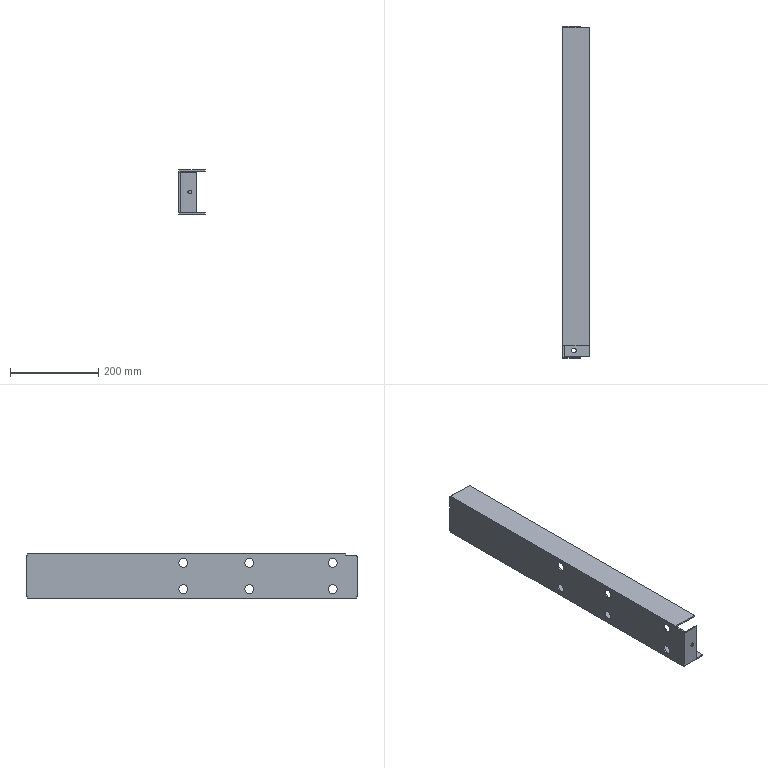Part | SolidWorks | features BaseBody 1 | 1 solid | 44 faces | box 60 x 754 x 100 mm | volume 491228 mm3 | plane 24 | cylinder 20 | commonest cylinder face diameters 20 x12 11 x4 8.5 x2 10.6 x2
STEP:
#1=CARTESIAN_POINT('',(199.946,-4340.973,914.971));
#2=VERTEX_POINT('',#1);
#3=CARTESIAN_POINT('',(199.946,-4340.973,934.971));
#4=VERTEX_POINT('',#3);
#5=CARTESIAN_POINT('',(199.946,-4340.973,924.971));
#6=DIRECTION('',(-1.,0.,0.));
#7=DIRECTION('',(0.,0.,1.));
#8=AXIS2_PLACEMENT_3D('',#5,#6,#7);
#9=CIRCLE('',#8,10.);
#10=EDGE_CURVE('',#2,#4,#9,.T.);
#11=ORIENTED_EDGE('',*,*,#10,.F.);
#12=CARTESIAN_POINT('',(196.946,-4340.973,914.971));
#13=VERTEX_POINT('',#12);
#14=CARTESIAN_POINT('',(218.146,-4340.973,914.971));
#15=DIRECTION('',(-1.,0.,0.));
#16=VECTOR('',#15,1000.);
#17=LINE('',#14,#16);
#18=EDGE_CURVE('',#2,#13,#17,.T.);
#19=ORIENTED_EDGE('',*,*,#18,.T.);
#20=CARTESIAN_POINT('',(196.946,-4340.973,934.971));
#21=VERTEX_POINT('',#20);
#22=CARTESIAN_POINT('',(196.946,-4340.973,924.971));
#23=DIRECTION('',(1.,0.,0.));
#24=DIRECTION('',(0.,0.,1.));
#25=AXIS2_PLACEMENT_3D('',#22,#23,#24);
#26=CIRCLE('',#25,10.);
#27=EDGE_CURVE('',#21,#13,#26,.T.);
#28=ORIENTED_EDGE('',*,*,#27,.F.);
#29=CARTESIAN_POINT('',(218.146,-4340.973,934.971));
#30=DIRECTION('',(-1.,0.,0.));
#31=VECTOR('',#30,1000.);
#32=LINE('',#29,#31);
#33=EDGE_CURVE('',#4,#21,#32,.T.);
#34=ORIENTED_EDGE('',*,*,#33,.F.);
#35=EDGE_LOOP('',(#11,#19,#28,#34));
#36=FACE_OUTER_BOUND('',#35,.T.);
#37=CARTESIAN_POINT('',(218.146,-4340.973,924.971));
#38=DIRECTION('',(-1.,0.,0.));
#39=DIRECTION('',(0.,0.,1.));
#40=AXIS2_PLACEMENT_3D('',#37,#38,#39);
#41=CYLINDRICAL_SURFACE('',#40,10.);
#42=ADVANCED_FACE('',(#36),#41,.F.);
#43=CARTESIAN_POINT('',(199.946,-4150.973,854.971));
#44=VERTEX_POINT('',#43);
#45=CARTESIAN_POINT('',(199.946,-4150.973,874.971));
#46=VERTEX_POINT('',#45);
#47=CARTESIAN_POINT('',(199.946,-4150.973,864.971));
#48=DIRECTION('',(-1.,0.,0.));
#49=DIRECTION('',(0.,0.,1.));
#50=AXIS2_PLACEMENT_3D('',#47,#48,#49);
#51=CIRCLE('',#50,10.);
#52=EDGE_CURVE('',#44,#46,#51,.T.);
#53=ORIENTED_EDGE('',*,*,#52,.F.);
#54=CARTESIAN_POINT('',(196.946,-4150.973,854.971));
#55=VERTEX_POINT('',#54);
#56=CARTESIAN_POINT('',(218.146,-4150.973,854.971));
#57=DIRECTION('',(-1.,0.,0.));
#58=VECTOR('',#57,1000.);
#59=LINE('',#56,#58);
#60=EDGE_CURVE('',#44,#55,#59,.T.);
#61=ORIENTED_EDGE('',*,*,#60,.T.);
#62=CARTESIAN_POINT('',(196.946,-4150.973,874.971));
#63=VERTEX_POINT('',#62);
#64=CARTESIAN_POINT('',(196.946,-4150.973,864.971));
#65=DIRECTION('',(1.,0.,0.));
#66=DIRECTION('',(0.,0.,1.));
#67=AXIS2_PLACEMENT_3D('',#64,#65,#66);
#68=CIRCLE('',#67,10.);
#69=EDGE_CURVE('',#63,#55,#68,.T.);
#70=ORIENTED_EDGE('',*,*,#69,.F.);
#71=CARTESIAN_POINT('',(218.146,-4150.973,874.971));
#72=DIRECTION('',(-1.,0.,0.));
#73=VECTOR('',#72,1000.);
#74=LINE('',#71,#73);
#75=EDGE_CURVE('',#46,#63,#74,.T.);
#76=ORIENTED_EDGE('',*,*,#75,.F.);
#77=EDGE_LOOP('',(#53,#61,#70,#76));
#78=FACE_OUTER_BOUND('',#77,.T.);
#79=CARTESIAN_POINT('',(218.146,-4150.973,864.971));
#80=DIRECTION('',(-1.,0.,0.));
#81=DIRECTION('',(0.,0.,1.));
#82=AXIS2_PLACEMENT_3D('',#79,#80,#81);
#83=CYLINDRICAL_SURFACE('',#82,10.);
#84=ADVANCED_FACE('',(#78),#83,.F.);
#85=CARTESIAN_POINT('',(199.946,-4000.973,914.971));
#86=VERTEX_POINT('',#85);
#87=CARTESIAN_POINT('',(199.946,-4000.973,934.971));
#88=VERTEX_POINT('',#87);
#89=CARTESIAN_POINT('',(199.946,-4000.973,924.971));
#90=DIRECTION('',(-1.,0.,0.));
#91=DIRECTION('',(0.,0.,1.));
#92=AXIS2_PLACEMENT_3D('',#89,#90,#91);
#93=CIRCLE('',#92,10.);
#94=EDGE_CURVE('',#86,#88,#93,.T.);
#95=ORIENTED_EDGE('',*,*,#94,.F.);
#96=CARTESIAN_POINT('',(196.946,-4000.973,914.971));
#97=VERTEX_POINT('',#96);
#98=CARTESIAN_POINT('',(218.146,-4000.973,914.971));
#99=DIRECTION('',(-1.,0.,0.));
#100=VECTOR('',#99,1000.);
#101=LINE('',#98,#100);
#102=EDGE_CURVE('',#86,#97,#101,.T.);
#103=ORIENTED_EDGE('',*,*,#102,.T.);
#104=CARTESIAN_POINT('',(196.946,-4000.973,934.971));
#105=VERTEX_POINT('',#104);
#106=CARTESIAN_POINT('',(196.946,-4000.973,924.971));
#107=DIRECTION('',(1.,0.,0.));
#108=DIRECTION('',(0.,0.,1.));
#109=AXIS2_PLACEMENT_3D('',#106,#107,#108);
#110=CIRCLE('',#109,10.);
#111=EDGE_CURVE('',#105,#97,#110,.T.);
#112=ORIENTED_EDGE('',*,*,#111,.F.);
#113=CARTESIAN_POINT('',(218.146,-4000.973,934.971));
#114=DIRECTION('',(-1.,0.,0.));
#115=VECTOR('',#114,1000.);
#116=LINE('',#113,#115);
#117=EDGE_CURVE('',#88,#105,#116,.T.);
#118=ORIENTED_EDGE('',*,*,#117,.F.);
#119=EDGE_LOOP('',(#95,#103,#112,#118));
#120=FACE_OUTER_BOUND('',#119,.T.);
#121=CARTESIAN_POINT('',(218.146,-4000.973,924.971));
#122=DIRECTION('',(-1.,0.,0.));
#123=DIRECTION('',(0.,0.,1.));
#124=AXIS2_PLACEMENT_3D('',#121,#122,#123);
#125=CYLINDRICAL_SURFACE('',#124,10.);
#126=ADVANCED_FACE('',(#120),#125,.F.);
#127=CARTESIAN_POINT('',(199.946,-4000.973,854.971));
#128=VERTEX_POINT('',#127);
#129=CARTESIAN_POINT('',(199.946,-4000.973,874.971));
#130=VERTEX_POINT('',#129);
#131=CARTESIAN_POINT('',(199.946,-4000.973,864.971));
#132=DIRECTION('',(-1.,0.,0.));
#133=DIRECTION('',(0.,0.,1.));
#134=AXIS2_PLACEMENT_3D('',#131,#132,#133);
#135=CIRCLE('',#134,10.);
#136=EDGE_CURVE('',#128,#130,#135,.T.);
#137=ORIENTED_EDGE('',*,*,#136,.F.);
#138=CARTESIAN_POINT('',(196.946,-4000.973,854.971));
#139=VERTEX_POINT('',#138);
#140=CARTESIAN_POINT('',(218.146,-4000.973,854.971));
#141=DIRECTION('',(-1.,0.,0.));
#142=VECTOR('',#141,1000.);
#143=LINE('',#140,#142);
#144=EDGE_CURVE('',#128,#139,#143,.T.);
#145=ORIENTED_EDGE('',*,*,#144,.T.);
#146=CARTESIAN_POINT('',(196.946,-4000.973,874.971));
#147=VERTEX_POINT('',#146);
#148=CARTESIAN_POINT('',(196.946,-4000.973,864.971));
#149=DIRECTION('',(1.,0.,0.));
#150=DIRECTION('',(0.,0.,1.));
#151=AXIS2_PLACEMENT_3D('',#148,#149,#150);
#152=CIRCLE('',#151,10.);
#153=EDGE_CURVE('',#147,#139,#152,.T.);
#154=ORIENTED_EDGE('',*,*,#153,.F.);
#155=CARTESIAN_POINT('',(218.146,-4000.973,874.971));
#156=DIRECTION('',(-1.,0.,0.));
#157=VECTOR('',#156,1000.);
#158=LINE('',#155,#157);
#159=EDGE_CURVE('',#130,#147,#158,.T.);
#160=ORIENTED_EDGE('',*,*,#159,.F.);
#161=EDGE_LOOP('',(#137,#145,#154,#160));
#162=FACE_OUTER_BOUND('',#161,.T.);
#163=CARTESIAN_POINT('',(218.146,-4000.973,864.971));
#164=DIRECTION('',(-1.,0.,0.));
#165=DIRECTION('',(0.,0.,1.));
#166=AXIS2_PLACEMENT_3D('',#163,#164,#165);
#167=CYLINDRICAL_SURFACE('',#166,10.);
#168=ADVANCED_FACE('',(#162),#167,.F.);
#169=CARTESIAN_POINT('',(199.946,-4150.973,914.971));
#170=VERTEX_POINT('',#169);
#171=CARTESIAN_POINT('',(199.946,-4150.973,934.971));
#172=VERTEX_POINT('',#171);
#173=CARTESIAN_POINT('',(199.946,-4150.973,924.971));
#174=DIRECTION('',(-1.,0.,0.));
#175=DIRECTION('',(0.,0.,1.));
#176=AXIS2_PLACEMENT_3D('',#173,#174,#175);
#177=CIRCLE('',#176,10.);
#178=EDGE_CURVE('',#170,#172,#177,.T.);
#179=ORIENTED_EDGE('',*,*,#178,.F.);
#180=CARTESIAN_POINT('',(196.946,-4150.973,914.971));
#181=VERTEX_POINT('',#180);
#182=CARTESIAN_POINT('',(218.146,-4150.973,914.971));
#183=DIRECTION('',(-1.,0.,0.));
#184=VECTOR('',#183,1000.);
#185=LINE('',#182,#184);
#186=EDGE_CURVE('',#170,#181,#185,.T.);
#187=ORIENTED_EDGE('',*,*,#186,.T.);
#188=CARTESIAN_POINT('',(196.946,-4150.973,934.971));
#189=VERTEX_POINT('',#188);
#190=CARTESIAN_POINT('',(196.946,-4150.973,924.971));
#191=DIRECTION('',(1.,0.,0.));
#192=DIRECTION('',(0.,0.,1.));
#193=AXIS2_PLACEMENT_3D('',#190,#191,#192);
#194=CIRCLE('',#193,10.);
#195=EDGE_CURVE('',#189,#181,#194,.T.);
#196=ORIENTED_EDGE('',*,*,#195,.F.);
#197=CARTESIAN_POINT('',(218.146,-4150.973,934.971));
#198=DIRECTION('',(-1.,0.,0.));
#199=VECTOR('',#198,1000.);
#200=LINE('',#197,#199);
#201=EDGE_CURVE('',#172,#189,#200,.T.);
#202=ORIENTED_EDGE('',*,*,#201,.F.);
#203=EDGE_LOOP('',(#179,#187,#196,#202));
#204=FACE_OUTER_BOUND('',#203,.T.);
#205=CARTESIAN_POINT('',(218.146,-4150.973,924.971));
#206=DIRECTION('',(-1.,0.,0.));
#207=DIRECTION('',(0.,0.,1.));
#208=AXIS2_PLACEMENT_3D('',#205,#206,#207);
#209=CYLINDRICAL_SURFACE('',#208,10.);
#210=ADVANCED_FACE('',(#204),#209,.F.);
#211=CARTESIAN_POINT('',(199.946,-4340.973,854.971));
#212=VERTEX_POINT('',#211);
#213=CARTESIAN_POINT('',(199.946,-4340.973,874.971));
#214=VERTEX_POINT('',#213);
#215=CARTESIAN_POINT('',(199.946,-4340.973,864.971));
#216=DIRECTION('',(-1.,0.,0.));
#217=DIRECTION('',(0.,0.,1.));
#218=AXIS2_PLACEMENT_3D('',#215,#216,#217);
#219=CIRCLE('',#218,10.);
#220=EDGE_CURVE('',#212,#214,#219,.T.);
#221=ORIENTED_EDGE('',*,*,#220,.F.);
#222=CARTESIAN_POINT('',(196.946,-4340.973,854.971));
#223=VERTEX_POINT('',#222);
#224=CARTESIAN_POINT('',(218.146,-4340.973,854.971));
#225=DIRECTION('',(-1.,0.,0.));
#226=VECTOR('',#225,1000.);
#227=LINE('',#224,#226);
#228=EDGE_CURVE('',#212,#223,#227,.T.);
#229=ORIENTED_EDGE('',*,*,#228,.T.);
#230=CARTESIAN_POINT('',(196.946,-4340.973,874.971));
#231=VERTEX_POINT('',#230);
#232=CARTESIAN_POINT('',(196.946,-4340.973,864.971));
#233=DIRECTION('',(1.,0.,0.));
#234=DIRECTION('',(0.,0.,1.));
#235=AXIS2_PLACEMENT_3D('',#232,#233,#234);
#236=CIRCLE('',#235,10.);
#237=EDGE_CURVE('',#231,#223,#236,.T.);
#238=ORIENTED_EDGE('',*,*,#237,.F.);
#239=CARTESIAN_POINT('',(218.146,-4340.973,874.971));
#240=DIRECTION('',(-1.,0.,0.));
#241=VECTOR('',#240,1000.);
#242=LINE('',#239,#241);
#243=EDGE_CURVE('',#214,#231,#242,.T.);
#244=ORIENTED_EDGE('',*,*,#243,.F.);
#245=EDGE_LOOP('',(#221,#229,#238,#244));
#246=FACE_OUTER_BOUND('',#245,.T.);
#247=CARTESIAN_POINT('',(218.146,-4340.973,864.971));
#248=DIRECTION('',(-1.,0.,0.));
#249=DIRECTION('',(0.,0.,1.));
#250=AXIS2_PLACEMENT_3D('',#247,#248,#249);
#251=CYLINDRICAL_SURFACE('',#250,10.);
#252=ADVANCED_FACE('',(#246),#251,.F.);
#253=CARTESIAN_POINT('',(221.946,-4394.973,899.221));
#254=VERTEX_POINT('',#253);
#255=CARTESIAN_POINT('',(221.946,-4394.973,890.721));
#256=VERTEX_POINT('',#255);
#257=CARTESIAN_POINT('',(221.946,-4394.973,894.971));
#258=DIRECTION('',(0.,-1.,0.));
#259=DIRECTION('',(0.,0.,-1.));
#260=AXIS2_PLACEMENT_3D('',#257,#258,#259);
#261=CIRCLE('',#260,4.25);
#262=EDGE_CURVE('',#254,#256,#261,.T.);
#263=ORIENTED_EDGE('',*,*,#262,.F.);
#264=CARTESIAN_POINT('',(221.946,-4397.973,899.221));
#265=VERTEX_POINT('',#264);
#266=CARTESIAN_POINT('',(221.946,-4409.781,899.221));
#267=DIRECTION('',(0.,-1.,0.));
#268=VECTOR('',#267,1000.);
#269=LINE('',#266,#268);
#270=EDGE_CURVE('',#254,#265,#269,.T.);
#271=ORIENTED_EDGE('',*,*,#270,.T.);
#272=CARTESIAN_POINT('',(221.946,-4397.973,890.721));
#273=VERTEX_POINT('',#272);
#274=CARTESIAN_POINT('',(221.946,-4397.973,894.971));
#275=DIRECTION('',(0.,1.,0.));
#276=DIRECTION('',(0.,0.,-1.));
#277=AXIS2_PLACEMENT_3D('',#274,#275,#276);
#278=CIRCLE('',#277,4.25);
#279=EDGE_CURVE('',#273,#265,#278,.T.);
#280=ORIENTED_EDGE('',*,*,#279,.F.);
#281=CARTESIAN_POINT('',(221.946,-4409.781,890.721));
#282=DIRECTION('',(0.,-1.,0.));
#283=VECTOR('',#282,1000.);
#284=LINE('',#281,#283);
#285=EDGE_CURVE('',#256,#273,#284,.T.);
#286=ORIENTED_EDGE('',*,*,#285,.F.);
#287=EDGE_LOOP('',(#263,#271,#280,#286));
#288=FACE_OUTER_BOUND('',#287,.T.);
#289=CARTESIAN_POINT('',(221.946,-4409.781,894.971));
#290=DIRECTION('',(0.,-1.,0.));
#291=DIRECTION('',(0.,0.,-1.));
#292=AXIS2_PLACEMENT_3D('',#289,#290,#291);
#293=CYLINDRICAL_SURFACE('',#292,4.25);
#294=ADVANCED_FACE('',(#288),#293,.F.);
#295=CARTESIAN_POINT('',(216.646,-4380.973,844.971));
#296=VERTEX_POINT('',#295);
#297=CARTESIAN_POINT('',(227.246,-4380.973,844.971));
#298=VERTEX_POINT('',#297);
#299=CARTESIAN_POINT('',(221.946,-4380.973,844.971));
#300=DIRECTION('',(0.,0.,1.));
#301=DIRECTION('',(1.,0.,0.));
#302=AXIS2_PLACEMENT_3D('',#299,#300,#301);
#303=CIRCLE('',#302,5.3);
#304=EDGE_CURVE('',#296,#298,#303,.T.);
#305=ORIENTED_EDGE('',*,*,#304,.F.);
#306=CARTESIAN_POINT('',(216.646,-4380.973,847.971));
#307=VERTEX_POINT('',#306);
#308=CARTESIAN_POINT('',(216.646,-4380.973,840.704));
#309=DIRECTION('',(0.,0.,1.));
#310=VECTOR('',#309,1000.);
#311=LINE('',#308,#310);
#312=EDGE_CURVE('',#296,#307,#311,.T.);
#313=ORIENTED_EDGE('',*,*,#312,.T.);
#314=CARTESIAN_POINT('',(227.246,-4380.973,847.971));
#315=VERTEX_POINT('',#314);
#316=CARTESIAN_POINT('',(221.946,-4380.973,847.971));
#317=DIRECTION('',(0.,0.,-1.));
#318=DIRECTION('',(1.,0.,0.));
#319=AXIS2_PLACEMENT_3D('',#316,#317,#318);
#320=CIRCLE('',#319,5.3);
#321=EDGE_CURVE('',#315,#307,#320,.T.);
#322=ORIENTED_EDGE('',*,*,#321,.F.);
#323=CARTESIAN_POINT('',(227.246,-4380.973,840.704));
#324=DIRECTION('',(0.,0.,1.));
#325=VECTOR('',#324,1000.);
#326=LINE('',#323,#325);
#327=EDGE_CURVE('',#298,#315,#326,.T.);
#328=ORIENTED_EDGE('',*,*,#327,.F.);
#329=EDGE_LOOP('',(#305,#313,#322,#328));
#330=FACE_OUTER_BOUND('',#329,.T.);
#331=CARTESIAN_POINT('',(221.946,-4380.973,840.704));
#332=DIRECTION('',(0.,0.,1.));
#333=DIRECTION('',(1.,0.,0.));
#334=AXIS2_PLACEMENT_3D('',#331,#332,#333);
#335=CYLINDRICAL_SURFACE('',#334,5.3);
#336=ADVANCED_FACE('',(#330),#335,.F.);
#337=CARTESIAN_POINT('',(221.946,-3643.973,930.471));
#338=VERTEX_POINT('',#337);
#339=CARTESIAN_POINT('',(221.946,-3643.973,919.471));
#340=VERTEX_POINT('',#339);
#341=CARTESIAN_POINT('',(221.946,-3643.973,924.971));
#342=DIRECTION('',(0.,-1.,0.));
#343=DIRECTION('',(0.,0.,-1.));
#344=AXIS2_PLACEMENT_3D('',#341,#342,#343);
#345=CIRCLE('',#344,5.5);
#346=EDGE_CURVE('',#338,#340,#345,.T.);
#347=ORIENTED_EDGE('',*,*,#346,.F.);
#348=CARTESIAN_POINT('',(221.946,-3646.973,930.471));
#349=VERTEX_POINT('',#348);
#350=CARTESIAN_POINT('',(221.946,-3631.308,930.471));
#351=DIRECTION('',(0.,-1.,0.));
#352=VECTOR('',#351,1000.);
#353=LINE('',#350,#352);
#354=EDGE_CURVE('',#338,#349,#353,.T.);
#355=ORIENTED_EDGE('',*,*,#354,.T.);
#356=CARTESIAN_POINT('',(221.946,-3646.973,919.471));
#357=VERTEX_POINT('',#356);
#358=CARTESIAN_POINT('',(221.946,-3646.973,924.971));
#359=DIRECTION('',(0.,-1.,0.));
#360=DIRECTION('',(0.,0.,-1.));
#361=AXIS2_PLACEMENT_3D('',#358,#359,#360);
#362=CIRCLE('',#361,5.5);
#363=EDGE_CURVE('',#349,#357,#362,.T.);
#364=ORIENTED_EDGE('',*,*,#363,.T.);
#365=CARTESIAN_POINT('',(221.946,-3631.308,919.471));
#366=DIRECTION('',(0.,-1.,0.));
#367=VECTOR('',#366,1000.);
#368=LINE('',#365,#367);
#369=EDGE_CURVE('',#340,#357,#368,.T.);
#370=ORIENTED_EDGE('',*,*,#369,.F.);
#371=EDGE_LOOP('',(#347,#355,#364,#370));
#372=FACE_OUTER_BOUND('',#371,.T.);
#373=CARTESIAN_POINT('',(221.946,-3631.308,924.971));
#374=DIRECTION('',(0.,-1.,0.));
#375=DIRECTION('',(0.,0.,-1.));
#376=AXIS2_PLACEMENT_3D('',#373,#374,#375);
#377=CYLINDRICAL_SURFACE('',#376,5.5);
#378=ADVANCED_FACE('',(#372),#377,.F.);
#379=CARTESIAN_POINT('',(221.946,-3643.973,870.471));
#380=VERTEX_POINT('',#379);
#381=CARTESIAN_POINT('',(221.946,-3643.973,859.471));
#382=VERTEX_POINT('',#381);
#383=CARTESIAN_POINT('',(221.946,-3643.973,864.971));
#384=DIRECTION('',(0.,-1.,0.));
#385=DIRECTION('',(0.,0.,-1.));
#386=AXIS2_PLACEMENT_3D('',#383,#384,#385);
#387=CIRCLE('',#386,5.5);
#388=EDGE_CURVE('',#380,#382,#387,.T.);
#389=ORIENTED_EDGE('',*,*,#388,.F.);
#390=CARTESIAN_POINT('',(221.946,-3646.973,870.471));
#391=VERTEX_POINT('',#390);
#392=CARTESIAN_POINT('',(221.946,-3631.308,870.471));
#393=DIRECTION('',(0.,-1.,0.));
#394=VECTOR('',#393,1000.);
#395=LINE('',#392,#394);
#396=EDGE_CURVE('',#380,#391,#395,.T.);
#397=ORIENTED_EDGE('',*,*,#396,.T.);
#398=CARTESIAN_POINT('',(221.946,-3646.973,859.471));
#399=VERTEX_POINT('',#398);
#400=CARTESIAN_POINT('',(221.946,-3646.973,864.971));
#401=DIRECTION('',(0.,-1.,0.));
#402=DIRECTION('',(0.,0.,-1.));
#403=AXIS2_PLACEMENT_3D('',#400,#401,#402);
#404=CIRCLE('',#403,5.5);
#405=EDGE_CURVE('',#391,#399,#404,.T.);
#406=ORIENTED_EDGE('',*,*,#405,.T.);
#407=CARTESIAN_POINT('',(221.946,-3631.308,859.471));
#408=DIRECTION('',(0.,-1.,0.));
#409=VECTOR('',#408,1000.);
#410=LINE('',#407,#409);
#411=EDGE_CURVE('',#382,#399,#410,.T.);
#412=ORIENTED_EDGE('',*,*,#411,.F.);
#413=EDGE_LOOP('',(#389,#397,#406,#412));
#414=FACE_OUTER_BOUND('',#413,.T.);
#415=CARTESIAN_POINT('',(221.946,-3631.308,864.971));
#416=DIRECTION('',(0.,-1.,0.));
#417=DIRECTION('',(0.,0.,-1.));
#418=AXIS2_PLACEMENT_3D('',#415,#416,#417);
#419=CYLINDRICAL_SURFACE('',#418,5.5);
#420=ADVANCED_FACE('',(#414),#419,.F.);
#421=CARTESIAN_POINT('',(196.946,-4394.973,848.021));
#422=VERTEX_POINT('',#421);
#423=CARTESIAN_POINT('',(196.946,-4397.973,848.021));
#424=VERTEX_POINT('',#423);
#425=CARTESIAN_POINT('',(196.946,-3643.973,848.021));
#426=DIRECTION('',(0.,-1.,0.));
#427=VECTOR('',#426,1000.);
#428=LINE('',#425,#427);
#429=EDGE_CURVE('',#422,#424,#428,.T.);
#430=ORIENTED_EDGE('',*,*,#429,.T.);
#431=CARTESIAN_POINT('',(196.946,-4397.973,938.921));
#432=VERTEX_POINT('',#431);
#433=CARTESIAN_POINT('',(196.946,-4397.973,868.021));
#434=DIRECTION('',(0.,0.,1.));
#435=VECTOR('',#434,1000.);
#436=LINE('',#433,#435);
#437=EDGE_CURVE('',#424,#432,#436,.T.);
#438=ORIENTED_EDGE('',*,*,#437,.T.);
#439=CARTESIAN_POINT('',(196.946,-4394.973,938.921));
#440=VERTEX_POINT('',#439);
#441=CARTESIAN_POINT('',(196.946,-3643.973,938.921));
#442=DIRECTION('',(0.,1.,0.));
#443=VECTOR('',#442,1000.);
#444=LINE('',#441,#443);
#445=EDGE_CURVE('',#432,#440,#444,.T.);
#446=ORIENTED_EDGE('',*,*,#445,.T.);
#447=CARTESIAN_POINT('',(196.946,-4394.973,941.921));
#448=VERTEX_POINT('',#447);
#449=CARTESIAN_POINT('',(196.946,-4394.973,868.021));
#450=DIRECTION('',(0.,0.,1.));
#451=VECTOR('',#450,1000.);
#452=LINE('',#449,#451);
#453=EDGE_CURVE('',#440,#448,#452,.T.);
#454=ORIENTED_EDGE('',*,*,#453,.T.);
#455=CARTESIAN_POINT('',(196.946,-4369.973,941.921));
#456=VERTEX_POINT('',#455);
#457=CARTESIAN_POINT('',(196.946,-3643.973,941.921));
#458=DIRECTION('',(0.,1.,0.));
#459=VECTOR('',#458,1000.);
#460=LINE('',#457,#459);
#461=EDGE_CURVE('',#448,#456,#460,.T.);
#462=ORIENTED_EDGE('',*,*,#461,.T.);
#463=CARTESIAN_POINT('',(196.946,-4369.973,944.971));
#464=VERTEX_POINT('',#463);
#465=CARTESIAN_POINT('',(196.946,-4369.973,868.021));
#466=DIRECTION('',(0.,0.,1.));
#467=VECTOR('',#466,1000.);
#468=LINE('',#465,#467);
#469=EDGE_CURVE('',#456,#464,#468,.T.);
#470=ORIENTED_EDGE('',*,*,#469,.T.);
#471=CARTESIAN_POINT('',(196.946,-3646.973,944.971));
#472=VERTEX_POINT('',#471);
#473=CARTESIAN_POINT('',(196.946,-3643.973,944.971));
#474=DIRECTION('',(0.,1.,0.));
#475=VECTOR('',#474,1000.);
#476=LINE('',#473,#475);
#477=EDGE_CURVE('',#464,#472,#476,.T.);
#478=ORIENTED_EDGE('',*,*,#477,.T.);
#479=CARTESIAN_POINT('',(196.946,-3646.973,941.921));
#480=VERTEX_POINT('',#479);
#481=CARTESIAN_POINT('',(196.946,-3646.973,868.021));
#482=DIRECTION('',(0.,0.,-1.));
#483=VECTOR('',#482,1000.);
#484=LINE('',#481,#483);
#485=EDGE_CURVE('',#472,#480,#484,.T.);
#486=ORIENTED_EDGE('',*,*,#485,.T.);
#487=CARTESIAN_POINT('',(196.946,-3643.973,941.921));
#488=VERTEX_POINT('',#487);
#489=CARTESIAN_POINT('',(196.946,-3643.973,941.921));
#490=DIRECTION('',(0.,1.,0.));
#491=VECTOR('',#490,1000.);
#492=LINE('',#489,#491);
#493=EDGE_CURVE('',#480,#488,#492,.T.);
#494=ORIENTED_EDGE('',*,*,#493,.T.);
#495=CARTESIAN_POINT('',(196.946,-3643.973,848.021));
#496=VERTEX_POINT('',#495);
#497=CARTESIAN_POINT('',(196.946,-3643.973,868.021));
#498=DIRECTION('',(0.,0.,-1.));
#499=VECTOR('',#498,1000.);
#500=LINE('',#497,#499);
#501=EDGE_CURVE('',#488,#496,#500,.T.);
#502=ORIENTED_EDGE('',*,*,#501,.T.);
#503=CARTESIAN_POINT('',(196.946,-3646.973,848.021));
#504=VERTEX_POINT('',#503);
#505=CARTESIAN_POINT('',(196.946,-3643.973,848.021));
#506=DIRECTION('',(0.,-1.,0.));
#507=VECTOR('',#506,1000.);
#508=LINE('',#505,#507);
#509=EDGE_CURVE('',#496,#504,#508,.T.);
#510=ORIENTED_EDGE('',*,*,#509,.T.);
#511=CARTESIAN_POINT('',(196.946,-3646.973,844.971));
#512=VERTEX_POINT('',#511);
#513=CARTESIAN_POINT('',(196.946,-3646.973,868.021));
#514=DIRECTION('',(0.,0.,-1.));
#515=VECTOR('',#514,1000.);
#516=LINE('',#513,#515);
#517=EDGE_CURVE('',#504,#512,#516,.T.);
#518=ORIENTED_EDGE('',*,*,#517,.T.);
#519=CARTESIAN_POINT('',(196.946,-4394.973,844.971));
#520=VERTEX_POINT('',#519);
#521=CARTESIAN_POINT('',(196.946,-3643.973,844.971));
#522=DIRECTION('',(0.,-1.,0.));
#523=VECTOR('',#522,1000.);
#524=LINE('',#521,#523);
#525=EDGE_CURVE('',#512,#520,#524,.T.);
#526=ORIENTED_EDGE('',*,*,#525,.T.);
#527=CARTESIAN_POINT('',(196.946,-4394.973,868.021));
#528=DIRECTION('',(0.,0.,1.));
#529=VECTOR('',#528,1000.);
#530=LINE('',#527,#529);
#531=EDGE_CURVE('',#520,#422,#530,.T.);
#532=ORIENTED_EDGE('',*,*,#531,.T.);
#533=EDGE_LOOP('',(#430,#438,#446,#454,#462,#470,#478,#486,#494,#502,#510,#518,#526,#532));
#534=FACE_OUTER_BOUND('',#533,.T.);
#535=ORIENTED_EDGE('',*,*,#27,.T.);
#536=CARTESIAN_POINT('',(196.946,-4340.973,924.971));
#537=DIRECTION('',(1.,0.,0.));
#538=DIRECTION('',(0.,0.,1.));
#539=AXIS2_PLACEMENT_3D('',#536,#537,#538);
#540=CIRCLE('',#539,10.);
#541=EDGE_CURVE('',#13,#21,#540,.T.);
#542=ORIENTED_EDGE('',*,*,#541,.T.);
#543=EDGE_LOOP('',(#535,#542));
#544=FACE_BOUND('',#543,.T.);
#545=ORIENTED_EDGE('',*,*,#69,.T.);
#546=CARTESIAN_POINT('',(196.946,-4150.973,864.971));
#547=DIRECTION('',(1.,0.,0.));
#548=DIRECTION('',(0.,0.,1.));
#549=AXIS2_PLACEMENT_3D('',#546,#547,#548);
#550=CIRCLE('',#549,10.);
#551=EDGE_CURVE('',#55,#63,#550,.T.);
#552=ORIENTED_EDGE('',*,*,#551,.T.);
#553=EDGE_LOOP('',(#545,#552));
#554=FACE_BOUND('',#553,.T.);
#555=ORIENTED_EDGE('',*,*,#111,.T.);
#556=CARTESIAN_POINT('',(196.946,-4000.973,924.971));
#557=DIRECTION('',(1.,0.,0.));
#558=DIRECTION('',(0.,0.,1.));
#559=AXIS2_PLACEMENT_3D('',#556,#557,#558);
#560=CIRCLE('',#559,10.);
#561=EDGE_CURVE('',#97,#105,#560,.T.);
#562=ORIENTED_EDGE('',*,*,#561,.T.);
#563=EDGE_LOOP('',(#555,#562));
#564=FACE_BOUND('',#563,.T.);
#565=ORIENTED_EDGE('',*,*,#153,.T.);
#566=CARTESIAN_POINT('',(196.946,-4000.973,864.971));
#567=DIRECTION('',(1.,0.,0.));
#568=DIRECTION('',(0.,0.,1.));
#569=AXIS2_PLACEMENT_3D('',#566,#567,#568);
#570=CIRCLE('',#569,10.);
#571=EDGE_CURVE('',#139,#147,#570,.T.);
#572=ORIENTED_EDGE('',*,*,#571,.T.);
#573=EDGE_LOOP('',(#565,#572));
#574=FACE_BOUND('',#573,.T.);
#575=ORIENTED_EDGE('',*,*,#195,.T.);
#576=CARTESIAN_POINT('',(196.946,-4150.973,924.971));
#577=DIRECTION('',(1.,0.,0.));
#578=DIRECTION('',(0.,0.,1.));
#579=AXIS2_PLACEMENT_3D('',#576,#577,#578);
#580=CIRCLE('',#579,10.);
#581=EDGE_CURVE('',#181,#189,#580,.T.);
#582=ORIENTED_EDGE('',*,*,#581,.T.);
#583=EDGE_LOOP('',(#575,#582));
#584=FACE_BOUND('',#583,.T.);
#585=ORIENTED_EDGE('',*,*,#237,.T.);
#586=CARTESIAN_POINT('',(196.946,-4340.973,864.971));
#587=DIRECTION('',(1.,0.,0.));
#588=DIRECTION('',(0.,0.,1.));
#589=AXIS2_PLACEMENT_3D('',#586,#587,#588);
#590=CIRCLE('',#589,10.);
#591=EDGE_CURVE('',#223,#231,#590,.T.);
#592=ORIENTED_EDGE('',*,*,#591,.T.);
#593=EDGE_LOOP('',(#585,#592));
#594=FACE_BOUND('',#593,.T.);
#595=CARTESIAN_POINT('',(196.946,-3643.973,868.021));
#596=DIRECTION('',(-1.,0.,0.));
#597=DIRECTION('',(0.,0.,1.));
#598=AXIS2_PLACEMENT_3D('',#595,#596,#597);
#599=PLANE('',#598);
#600=ADVANCED_FACE('',(#534,#544,#554,#564,#574,#584,#594),#599,.T.);
#601=CARTESIAN_POINT('',(236.946,-4397.973,848.021));
#602=VERTEX_POINT('',#601);
#603=CARTESIAN_POINT('',(216.946,-4397.973,848.021));
#604=DIRECTION('',(1.,0.,0.));
#605=VECTOR('',#604,1000.);
#606=LINE('',#603,#605);
#607=EDGE_CURVE('',#424,#602,#606,.T.);
#608=ORIENTED_EDGE('',*,*,#607,.T.);
#609=CARTESIAN_POINT('',(236.946,-4397.973,938.921));
#610=VERTEX_POINT('',#609);
#611=CARTESIAN_POINT('',(236.946,-4397.973,904.971));
#612=DIRECTION('',(0.,0.,1.));
#613=VECTOR('',#612,1000.);
#614=LINE('',#611,#613);
#615=EDGE_CURVE('',#602,#610,#614,.T.);
#616=ORIENTED_EDGE('',*,*,#615,.T.);
#617=CARTESIAN_POINT('',(216.946,-4397.973,938.921));
#618=DIRECTION('',(-1.,0.,0.));
#619=VECTOR('',#618,1000.);
#620=LINE('',#617,#619);
#621=EDGE_CURVE('',#610,#432,#620,.T.);
#622=ORIENTED_EDGE('',*,*,#621,.T.);
#623=ORIENTED_EDGE('',*,*,#437,.F.);
#624=EDGE_LOOP('',(#608,#616,#622,#623));
#625=FACE_OUTER_BOUND('',#624,.T.);
#626=ORIENTED_EDGE('',*,*,#279,.T.);
#627=CARTESIAN_POINT('',(221.946,-4397.973,894.971));
#628=DIRECTION('',(0.,1.,0.));
#629=DIRECTION('',(0.,0.,-1.));
#630=AXIS2_PLACEMENT_3D('',#627,#628,#629);
#631=CIRCLE('',#630,4.25);
#632=EDGE_CURVE('',#265,#273,#631,.T.);
#633=ORIENTED_EDGE('',*,*,#632,.T.);
#634=EDGE_LOOP('',(#626,#633));
#635=FACE_BOUND('',#634,.T.);
#636=CARTESIAN_POINT('',(216.946,-4397.973,904.971));
#637=DIRECTION('',(0.,-1.,0.));
#638=DIRECTION('',(0.,0.,-1.));
#639=AXIS2_PLACEMENT_3D('',#636,#637,#638);
#640=PLANE('',#639);
#641=ADVANCED_FACE('',(#625,#635),#640,.T.);
#642=ORIENTED_EDGE('',*,*,#607,.F.);
#643=ORIENTED_EDGE('',*,*,#429,.F.);
#644=CARTESIAN_POINT('',(199.946,-4394.973,848.021));
#645=VERTEX_POINT('',#644);
#646=CARTESIAN_POINT('',(236.946,-4394.973,848.021));
#647=DIRECTION('',(1.,0.,0.));
#648=VECTOR('',#647,1000.);
#649=LINE('',#646,#648);
#650=EDGE_CURVE('',#422,#645,#649,.T.);
#651=ORIENTED_EDGE('',*,*,#650,.T.);
#652=CARTESIAN_POINT('',(236.946,-4394.973,848.021));
#653=VERTEX_POINT('',#652);
#654=CARTESIAN_POINT('',(236.946,-4394.973,848.021));
#655=DIRECTION('',(1.,0.,0.));
#656=VECTOR('',#655,1000.);
#657=LINE('',#654,#656);
#658=EDGE_CURVE('',#645,#653,#657,.T.);
#659=ORIENTED_EDGE('',*,*,#658,.T.);
#660=CARTESIAN_POINT('',(236.946,-4398.973,848.021));
#661=DIRECTION('',(0.,-1.,0.));
#662=VECTOR('',#661,1000.);
#663=LINE('',#660,#662);
#664=EDGE_CURVE('',#653,#602,#663,.T.);
#665=ORIENTED_EDGE('',*,*,#664,.T.);
#666=EDGE_LOOP('',(#642,#643,#651,#659,#665));
#667=FACE_OUTER_BOUND('',#666,.T.);
#668=CARTESIAN_POINT('',(236.946,-4398.973,848.021));
#669=DIRECTION('',(0.,0.,-1.));
#670=DIRECTION('',(-1.,0.,0.));
#671=AXIS2_PLACEMENT_3D('',#668,#669,#670);
#672=PLANE('',#671);
#673=ADVANCED_FACE('',(#667),#672,.T.);
#674=CARTESIAN_POINT('',(256.946,-4394.973,847.971));
#675=VERTEX_POINT('',#674);
#676=CARTESIAN_POINT('',(199.946,-4394.973,847.971));
#677=VERTEX_POINT('',#676);
#678=CARTESIAN_POINT('',(216.674,-4394.973,847.971));
#679=DIRECTION('',(-1.,0.,0.));
#680=VECTOR('',#679,1000.);
#681=LINE('',#678,#680);
#682=EDGE_CURVE('',#675,#677,#681,.T.);
#683=ORIENTED_EDGE('',*,*,#682,.T.);
#684=CARTESIAN_POINT('',(199.946,-4394.973,941.971));
#685=DIRECTION('',(0.,0.,-1.));
#686=VECTOR('',#685,1000.);
#687=LINE('',#684,#686);
#688=EDGE_CURVE('',#645,#677,#687,.T.);
#689=ORIENTED_EDGE('',*,*,#688,.F.);
#690=ORIENTED_EDGE('',*,*,#650,.F.);
#691=ORIENTED_EDGE('',*,*,#531,.F.);
#692=CARTESIAN_POINT('',(256.946,-4394.973,844.971));
#693=VERTEX_POINT('',#692);
#694=CARTESIAN_POINT('',(216.674,-4394.973,844.971));
#695=DIRECTION('',(1.,0.,0.));
#696=VECTOR('',#695,1000.);
#697=LINE('',#694,#696);
#698=EDGE_CURVE('',#520,#693,#697,.T.);
#699=ORIENTED_EDGE('',*,*,#698,.T.);
#700=CARTESIAN_POINT('',(256.946,-4394.973,884.971));
#701=DIRECTION('',(0.,0.,1.));
#702=VECTOR('',#701,1000.);
#703=LINE('',#700,#702);
#704=EDGE_CURVE('',#693,#675,#703,.T.);
#705=ORIENTED_EDGE('',*,*,#704,.T.);
#706=EDGE_LOOP('',(#683,#689,#690,#691,#699,#705));
#707=FACE_OUTER_BOUND('',#706,.T.);
#708=CARTESIAN_POINT('',(216.674,-4394.973,884.971));
#709=DIRECTION('',(0.,-1.,0.));
#710=DIRECTION('',(0.,0.,-1.));
#711=AXIS2_PLACEMENT_3D('',#708,#709,#710);
#712=PLANE('',#711);
#713=ADVANCED_FACE('',(#707),#712,.T.);
#714=ORIENTED_EDGE('',*,*,#698,.F.);
#715=ORIENTED_EDGE('',*,*,#525,.F.);
#716=CARTESIAN_POINT('',(256.946,-3646.973,844.971));
#717=VERTEX_POINT('',#716);
#718=CARTESIAN_POINT('',(256.946,-3646.973,844.971));
#719=DIRECTION('',(1.,0.,0.));
#720=VECTOR('',#719,1000.);
#721=LINE('',#718,#720);
#722=EDGE_CURVE('',#512,#717,#721,.T.);
#723=ORIENTED_EDGE('',*,*,#722,.T.);
#724=CARTESIAN_POINT('',(256.946,-4398.973,844.971));
#725=DIRECTION('',(0.,-1.,0.));
#726=VECTOR('',#725,1000.);
#727=LINE('',#724,#726);
#728=EDGE_CURVE('',#717,#693,#727,.T.);
#729=ORIENTED_EDGE('',*,*,#728,.T.);
#730=EDGE_LOOP('',(#714,#715,#723,#729));
#731=FACE_OUTER_BOUND('',#730,.T.);
#732=CARTESIAN_POINT('',(221.946,-4380.973,844.971));
#733=DIRECTION('',(0.,0.,1.));
#734=DIRECTION('',(1.,0.,0.));
#735=AXIS2_PLACEMENT_3D('',#732,#733,#734);
#736=CIRCLE('',#735,5.3);
#737=EDGE_CURVE('',#298,#296,#736,.T.);
#738=ORIENTED_EDGE('',*,*,#737,.T.);
#739=ORIENTED_EDGE('',*,*,#304,.T.);
#740=EDGE_LOOP('',(#738,#739));
#741=FACE_BOUND('',#740,.T.);
#742=CARTESIAN_POINT('',(256.946,-4398.973,844.971));
#743=DIRECTION('',(0.,0.,-1.));
#744=DIRECTION('',(-1.,0.,0.));
#745=AXIS2_PLACEMENT_3D('',#742,#743,#744);
#746=PLANE('',#745);
#747=ADVANCED_FACE('',(#731,#741),#746,.T.);
#748=CARTESIAN_POINT('',(199.946,-3646.973,847.971));
#749=VERTEX_POINT('',#748);
#750=CARTESIAN_POINT('',(199.946,-3646.973,848.021));
#751=VERTEX_POINT('',#750);
#752=CARTESIAN_POINT('',(199.946,-3646.973,941.971));
#753=DIRECTION('',(0.,0.,1.));
#754=VECTOR('',#753,1000.);
#755=LINE('',#752,#754);
#756=EDGE_CURVE('',#749,#751,#755,.T.);
#757=ORIENTED_EDGE('',*,*,#756,.F.);
#758=CARTESIAN_POINT('',(256.946,-3646.973,847.971));
#759=VERTEX_POINT('',#758);
#760=CARTESIAN_POINT('',(216.674,-3646.973,847.971));
#761=DIRECTION('',(-1.,0.,0.));
#762=VECTOR('',#761,1000.);
#763=LINE('',#760,#762);
#764=EDGE_CURVE('',#759,#749,#763,.T.);
#765=ORIENTED_EDGE('',*,*,#764,.F.);
#766=CARTESIAN_POINT('',(256.946,-3646.973,904.971));
#767=DIRECTION('',(0.,0.,1.));
#768=VECTOR('',#767,1000.);
#769=LINE('',#766,#768);
#770=EDGE_CURVE('',#717,#759,#769,.T.);
#771=ORIENTED_EDGE('',*,*,#770,.F.);
#772=ORIENTED_EDGE('',*,*,#722,.F.);
#773=ORIENTED_EDGE('',*,*,#517,.F.);
#774=CARTESIAN_POINT('',(216.674,-3646.973,848.021));
#775=DIRECTION('',(-1.,0.,0.));
#776=VECTOR('',#775,1000.);
#777=LINE('',#774,#776);
#778=EDGE_CURVE('',#751,#504,#777,.T.);
#779=ORIENTED_EDGE('',*,*,#778,.F.);
#780=EDGE_LOOP('',(#757,#765,#771,#772,#773,#779));
#781=FACE_OUTER_BOUND('',#780,.T.);
#782=CARTESIAN_POINT('',(216.674,-3646.973,904.971));
#783=DIRECTION('',(0.,-1.,0.));
#784=DIRECTION('',(0.,0.,-1.));
#785=AXIS2_PLACEMENT_3D('',#782,#783,#784);
#786=PLANE('',#785);
#787=ADVANCED_FACE('',(#781),#786,.F.);
#788=CARTESIAN_POINT('',(236.946,-3643.973,848.021));
#789=VERTEX_POINT('',#788);
#790=CARTESIAN_POINT('',(236.946,-3643.973,848.021));
#791=DIRECTION('',(1.,0.,0.));
#792=VECTOR('',#791,1000.);
#793=LINE('',#790,#792);
#794=EDGE_CURVE('',#496,#789,#793,.T.);
#795=ORIENTED_EDGE('',*,*,#794,.T.);
#796=CARTESIAN_POINT('',(236.946,-3646.973,848.021));
#797=VERTEX_POINT('',#796);
#798=CARTESIAN_POINT('',(236.946,-3643.973,848.021));
#799=DIRECTION('',(0.,-1.,0.));
#800=VECTOR('',#799,1000.);
#801=LINE('',#798,#800);
#802=EDGE_CURVE('',#789,#797,#801,.T.);
#803=ORIENTED_EDGE('',*,*,#802,.T.);
#804=CARTESIAN_POINT('',(236.946,-3646.973,848.021));
#805=DIRECTION('',(-1.,0.,0.));
#806=VECTOR('',#805,1000.);
#807=LINE('',#804,#806);
#808=EDGE_CURVE('',#797,#751,#807,.T.);
#809=ORIENTED_EDGE('',*,*,#808,.T.);
#810=ORIENTED_EDGE('',*,*,#778,.T.);
#811=ORIENTED_EDGE('',*,*,#509,.F.);
#812=EDGE_LOOP('',(#795,#803,#809,#810,#811));
#813=FACE_OUTER_BOUND('',#812,.T.);
#814=CARTESIAN_POINT('',(236.946,-3643.973,848.021));
#815=DIRECTION('',(0.,0.,-1.));
#816=DIRECTION('',(-1.,0.,0.));
#817=AXIS2_PLACEMENT_3D('',#814,#815,#816);
#818=PLANE('',#817);
#819=ADVANCED_FACE('',(#813),#818,.T.);
#820=CARTESIAN_POINT('',(236.946,-3643.973,941.921));
#821=VERTEX_POINT('',#820);
#822=CARTESIAN_POINT('',(216.946,-3643.973,941.921));
#823=DIRECTION('',(1.,0.,0.));
#824=VECTOR('',#823,1000.);
#825=LINE('',#822,#824);
#826=EDGE_CURVE('',#488,#821,#825,.T.);
#827=ORIENTED_EDGE('',*,*,#826,.T.);
#828=CARTESIAN_POINT('',(236.946,-3643.973,904.971));
#829=DIRECTION('',(0.,0.,-1.));
#830=VECTOR('',#829,1000.);
#831=LINE('',#828,#830);
#832=EDGE_CURVE('',#821,#789,#831,.T.);
#833=ORIENTED_EDGE('',*,*,#832,.T.);
#834=ORIENTED_EDGE('',*,*,#794,.F.);
#835=ORIENTED_EDGE('',*,*,#501,.F.);
#836=EDGE_LOOP('',(#827,#833,#834,#835));
#837=FACE_OUTER_BOUND('',#836,.T.);
#838=CARTESIAN_POINT('',(221.946,-3643.973,924.971));
#839=DIRECTION('',(0.,-1.,0.));
#840=DIRECTION('',(0.,0.,-1.));
#841=AXIS2_PLACEMENT_3D('',#838,#839,#840);
#842=CIRCLE('',#841,5.5);
#843=EDGE_CURVE('',#340,#338,#842,.T.);
#844=ORIENTED_EDGE('',*,*,#843,.T.);
#845=ORIENTED_EDGE('',*,*,#346,.T.);
#846=EDGE_LOOP('',(#844,#845));
#847=FACE_BOUND('',#846,.T.);
#848=CARTESIAN_POINT('',(221.946,-3643.973,864.971));
#849=DIRECTION('',(0.,-1.,0.));
#850=DIRECTION('',(0.,0.,-1.));
#851=AXIS2_PLACEMENT_3D('',#848,#849,#850);
#852=CIRCLE('',#851,5.5);
#853=EDGE_CURVE('',#382,#380,#852,.T.);
#854=ORIENTED_EDGE('',*,*,#853,.T.);
#855=ORIENTED_EDGE('',*,*,#388,.T.);
#856=EDGE_LOOP('',(#854,#855));
#857=FACE_BOUND('',#856,.T.);
#858=CARTESIAN_POINT('',(216.946,-3643.973,904.971));
#859=DIRECTION('',(0.,1.,0.));
#860=DIRECTION('',(0.,0.,1.));
#861=AXIS2_PLACEMENT_3D('',#858,#859,#860);
#862=PLANE('',#861);
#863=ADVANCED_FACE('',(#837,#847,#857),#862,.T.);
#864=ORIENTED_EDGE('',*,*,#826,.F.);
#865=ORIENTED_EDGE('',*,*,#493,.F.);
#866=CARTESIAN_POINT('',(199.946,-3646.973,941.921));
#867=VERTEX_POINT('',#866);
#868=CARTESIAN_POINT('',(196.946,-3646.973,941.921));
#869=DIRECTION('',(1.,0.,0.));
#870=VECTOR('',#869,1000.);
#871=LINE('',#868,#870);
#872=EDGE_CURVE('',#480,#867,#871,.T.);
#873=ORIENTED_EDGE('',*,*,#872,.T.);
#874=CARTESIAN_POINT('',(236.946,-3646.973,941.921));
#875=VERTEX_POINT('',#874);
#876=CARTESIAN_POINT('',(196.946,-3646.973,941.921));
#877=DIRECTION('',(1.,0.,0.));
#878=VECTOR('',#877,1000.);
#879=LINE('',#876,#878);
#880=EDGE_CURVE('',#867,#875,#879,.T.);
#881=ORIENTED_EDGE('',*,*,#880,.T.);
#882=CARTESIAN_POINT('',(236.946,-3643.973,941.921));
#883=DIRECTION('',(0.,1.,0.));
#884=VECTOR('',#883,1000.);
#885=LINE('',#882,#884);
#886=EDGE_CURVE('',#875,#821,#885,.T.);
#887=ORIENTED_EDGE('',*,*,#886,.T.);
#888=EDGE_LOOP('',(#864,#865,#873,#881,#887));
#889=FACE_OUTER_BOUND('',#888,.T.);
#890=CARTESIAN_POINT('',(196.946,-3643.973,941.921));
#891=DIRECTION('',(0.,0.,1.));
#892=DIRECTION('',(1.,0.,0.));
#893=AXIS2_PLACEMENT_3D('',#890,#891,#892);
#894=PLANE('',#893);
#895=ADVANCED_FACE('',(#889),#894,.T.);
#896=ORIENTED_EDGE('',*,*,#485,.F.);
#897=CARTESIAN_POINT('',(256.946,-3646.973,944.971));
#898=VERTEX_POINT('',#897);
#899=CARTESIAN_POINT('',(216.674,-3646.973,944.971));
#900=DIRECTION('',(-1.,0.,0.));
#901=VECTOR('',#900,1000.);
#902=LINE('',#899,#901);
#903=EDGE_CURVE('',#898,#472,#902,.T.);
#904=ORIENTED_EDGE('',*,*,#903,.F.);
#905=CARTESIAN_POINT('',(256.946,-3646.973,941.971));
#906=VERTEX_POINT('',#905);
#907=CARTESIAN_POINT('',(256.946,-3646.973,904.971));
#908=DIRECTION('',(0.,0.,1.));
#909=VECTOR('',#908,1000.);
#910=LINE('',#907,#909);
#911=EDGE_CURVE('',#906,#898,#910,.T.);
#912=ORIENTED_EDGE('',*,*,#911,.F.);
#913=CARTESIAN_POINT('',(199.946,-3646.973,941.971));
#914=VERTEX_POINT('',#913);
#915=CARTESIAN_POINT('',(216.674,-3646.973,941.971));
#916=DIRECTION('',(1.,0.,0.));
#917=VECTOR('',#916,1000.);
#918=LINE('',#915,#917);
#919=EDGE_CURVE('',#914,#906,#918,.T.);
#920=ORIENTED_EDGE('',*,*,#919,.F.);
#921=CARTESIAN_POINT('',(199.946,-3646.973,941.971));
#922=DIRECTION('',(0.,0.,1.));
#923=VECTOR('',#922,1000.);
#924=LINE('',#921,#923);
#925=EDGE_CURVE('',#867,#914,#924,.T.);
#926=ORIENTED_EDGE('',*,*,#925,.F.);
#927=ORIENTED_EDGE('',*,*,#872,.F.);
#928=EDGE_LOOP('',(#896,#904,#912,#920,#926,#927));
#929=FACE_OUTER_BOUND('',#928,.T.);
#930=CARTESIAN_POINT('',(216.674,-3646.973,904.971));
#931=DIRECTION('',(0.,-1.,0.));
#932=DIRECTION('',(0.,0.,-1.));
#933=AXIS2_PLACEMENT_3D('',#930,#931,#932);
#934=PLANE('',#933);
#935=ADVANCED_FACE('',(#929),#934,.F.);
#936=CARTESIAN_POINT('',(256.946,-4369.973,944.971));
#937=VERTEX_POINT('',#936);
#938=CARTESIAN_POINT('',(196.946,-4369.973,944.971));
#939=DIRECTION('',(1.,0.,0.));
#940=VECTOR('',#939,1000.);
#941=LINE('',#938,#940);
#942=EDGE_CURVE('',#464,#937,#941,.T.);
#943=ORIENTED_EDGE('',*,*,#942,.T.);
#944=CARTESIAN_POINT('',(256.946,-4398.973,944.971));
#945=DIRECTION('',(0.,1.,0.));
#946=VECTOR('',#945,1000.);
#947=LINE('',#944,#946);
#948=EDGE_CURVE('',#937,#898,#947,.T.);
#949=ORIENTED_EDGE('',*,*,#948,.T.);
#950=ORIENTED_EDGE('',*,*,#903,.T.);
#951=ORIENTED_EDGE('',*,*,#477,.F.);
#952=EDGE_LOOP('',(#943,#949,#950,#951));
#953=FACE_OUTER_BOUND('',#952,.T.);
#954=CARTESIAN_POINT('',(196.946,-4398.973,944.971));
#955=DIRECTION('',(0.,0.,1.));
#956=DIRECTION('',(1.,0.,0.));
#957=AXIS2_PLACEMENT_3D('',#954,#955,#956);
#958=PLANE('',#957);
#959=ADVANCED_FACE('',(#953),#958,.T.);
#960=CARTESIAN_POINT('',(256.946,-4369.973,941.971));
#961=VERTEX_POINT('',#960);
#962=CARTESIAN_POINT('',(256.946,-4369.973,904.971));
#963=DIRECTION('',(0.,0.,1.));
#964=VECTOR('',#963,1000.);
#965=LINE('',#962,#964);
#966=EDGE_CURVE('',#961,#937,#965,.T.);
#967=ORIENTED_EDGE('',*,*,#966,.T.);
#968=ORIENTED_EDGE('',*,*,#942,.F.);
#969=ORIENTED_EDGE('',*,*,#469,.F.);
#970=CARTESIAN_POINT('',(199.946,-4369.973,941.921));
#971=VERTEX_POINT('',#970);
#972=CARTESIAN_POINT('',(216.674,-4369.973,941.921));
#973=DIRECTION('',(1.,0.,0.));
#974=VECTOR('',#973,1000.);
#975=LINE('',#972,#974);
#976=EDGE_CURVE('',#456,#971,#975,.T.);
#977=ORIENTED_EDGE('',*,*,#976,.T.);
#978=CARTESIAN_POINT('',(199.946,-4369.973,941.971));
#979=VERTEX_POINT('',#978);
#980=CARTESIAN_POINT('',(199.946,-4369.973,941.971));
#981=DIRECTION('',(0.,0.,-1.));
#982=VECTOR('',#981,1000.);
#983=LINE('',#980,#982);
#984=EDGE_CURVE('',#979,#971,#983,.T.);
#985=ORIENTED_EDGE('',*,*,#984,.F.);
#986=CARTESIAN_POINT('',(216.674,-4369.973,941.971));
#987=DIRECTION('',(1.,0.,0.));
#988=VECTOR('',#987,1000.);
#989=LINE('',#986,#988);
#990=EDGE_CURVE('',#979,#961,#989,.T.);
#991=ORIENTED_EDGE('',*,*,#990,.T.);
#992=EDGE_LOOP('',(#967,#968,#969,#977,#985,#991));
#993=FACE_OUTER_BOUND('',#992,.T.);
#994=CARTESIAN_POINT('',(216.674,-4369.973,904.971));
#995=DIRECTION('',(0.,-1.,0.));
#996=DIRECTION('',(0.,0.,-1.));
#997=AXIS2_PLACEMENT_3D('',#994,#995,#996);
#998=PLANE('',#997);
#999=ADVANCED_FACE('',(#993),#998,.T.);
#1000=ORIENTED_EDGE('',*,*,#976,.F.);
#1001=ORIENTED_EDGE('',*,*,#461,.F.);
#1002=CARTESIAN_POINT('',(199.946,-4394.973,941.921));
#1003=VERTEX_POINT('',#1002);
#1004=CARTESIAN_POINT('',(196.946,-4394.973,941.921));
#1005=DIRECTION('',(1.,0.,0.));
#1006=VECTOR('',#1005,1000.);
#1007=LINE('',#1004,#1006);
#1008=EDGE_CURVE('',#448,#1003,#1007,.T.);
#1009=ORIENTED_EDGE('',*,*,#1008,.T.);
#1010=CARTESIAN_POINT('',(199.946,-4398.973,941.921));
#1011=DIRECTION('',(0.,1.,0.));
#1012=VECTOR('',#1011,1000.);
#1013=LINE('',#1010,#1012);
#1014=EDGE_CURVE('',#1003,#971,#1013,.T.);
#1015=ORIENTED_EDGE('',*,*,#1014,.T.);
#1016=EDGE_LOOP('',(#1000,#1001,#1009,#1015));
#1017=FACE_OUTER_BOUND('',#1016,.T.);
#1018=CARTESIAN_POINT('',(196.946,-4398.973,941.921));
#1019=DIRECTION('',(0.,0.,1.));
#1020=DIRECTION('',(1.,0.,0.));
#1021=AXIS2_PLACEMENT_3D('',#1018,#1019,#1020);
#1022=PLANE('',#1021);
#1023=ADVANCED_FACE('',(#1017),#1022,.T.);
#1024=CARTESIAN_POINT('',(199.946,-4394.973,938.921));
#1025=VERTEX_POINT('',#1024);
#1026=CARTESIAN_POINT('',(-197.193,-4394.973,938.921));
#1027=DIRECTION('',(-1.,0.,0.));
#1028=VECTOR('',#1027,1000.);
#1029=LINE('',#1026,#1028);
#1030=EDGE_CURVE('',#1025,#440,#1029,.T.);
#1031=ORIENTED_EDGE('',*,*,#1030,.F.);
#1032=CARTESIAN_POINT('',(199.946,-4394.973,938.921));
#1033=DIRECTION('',(0.,0.,-1.));
#1034=VECTOR('',#1033,1000.);
#1035=LINE('',#1032,#1034);
#1036=EDGE_CURVE('',#1003,#1025,#1035,.T.);
#1037=ORIENTED_EDGE('',*,*,#1036,.F.);
#1038=ORIENTED_EDGE('',*,*,#1008,.F.);
#1039=ORIENTED_EDGE('',*,*,#453,.F.);
#1040=EDGE_LOOP('',(#1031,#1037,#1038,#1039));
#1041=FACE_OUTER_BOUND('',#1040,.T.);
#1042=CARTESIAN_POINT('',(-197.193,-4394.973,938.921));
#1043=DIRECTION('',(0.,1.,0.));
#1044=DIRECTION('',(0.,0.,1.));
#1045=AXIS2_PLACEMENT_3D('',#1042,#1043,#1044);
#1046=PLANE('',#1045);
#1047=ADVANCED_FACE('',(#1041),#1046,.F.);
#1048=ORIENTED_EDGE('',*,*,#621,.F.);
#1049=CARTESIAN_POINT('',(236.946,-4394.973,938.921));
#1050=VERTEX_POINT('',#1049);
#1051=CARTESIAN_POINT('',(236.946,-4399.973,938.921));
#1052=DIRECTION('',(0.,-1.,0.));
#1053=VECTOR('',#1052,1000.);
#1054=LINE('',#1051,#1053);
#1055=EDGE_CURVE('',#1050,#610,#1054,.T.);
#1056=ORIENTED_EDGE('',*,*,#1055,.F.);
#1057=CARTESIAN_POINT('',(-197.193,-4394.973,938.921));
#1058=DIRECTION('',(1.,0.,0.));
#1059=VECTOR('',#1058,1000.);
#1060=LINE('',#1057,#1059);
#1061=EDGE_CURVE('',#1025,#1050,#1060,.T.);
#1062=ORIENTED_EDGE('',*,*,#1061,.F.);
#1063=ORIENTED_EDGE('',*,*,#1030,.T.);
#1064=ORIENTED_EDGE('',*,*,#445,.F.);
#1065=EDGE_LOOP('',(#1048,#1056,#1062,#1063,#1064));
#1066=FACE_OUTER_BOUND('',#1065,.T.);
#1067=CARTESIAN_POINT('',(-197.193,-4399.973,938.921));
#1068=DIRECTION('',(0.,0.,-1.));
#1069=DIRECTION('',(-1.,0.,0.));
#1070=AXIS2_PLACEMENT_3D('',#1067,#1068,#1069);
#1071=PLANE('',#1070);
#1072=ADVANCED_FACE('',(#1066),#1071,.F.);
#1073=ORIENTED_EDGE('',*,*,#18,.F.);
#1074=CARTESIAN_POINT('',(199.946,-4340.973,924.971));
#1075=DIRECTION('',(-1.,0.,0.));
#1076=DIRECTION('',(0.,0.,1.));
#1077=AXIS2_PLACEMENT_3D('',#1074,#1075,#1076);
#1078=CIRCLE('',#1077,10.);
#1079=EDGE_CURVE('',#4,#2,#1078,.T.);
#1080=ORIENTED_EDGE('',*,*,#1079,.F.);
#1081=ORIENTED_EDGE('',*,*,#33,.T.);
#1082=ORIENTED_EDGE('',*,*,#541,.F.);
#1083=EDGE_LOOP('',(#1073,#1080,#1081,#1082));
#1084=FACE_OUTER_BOUND('',#1083,.T.);
#1085=CARTESIAN_POINT('',(218.146,-4340.973,924.971));
#1086=DIRECTION('',(-1.,0.,0.));
#1087=DIRECTION('',(0.,0.,1.));
#1088=AXIS2_PLACEMENT_3D('',#1085,#1086,#1087);
#1089=CYLINDRICAL_SURFACE('',#1088,10.);
#1090=ADVANCED_FACE('',(#1084),#1089,.F.);
#1091=ORIENTED_EDGE('',*,*,#60,.F.);
#1092=CARTESIAN_POINT('',(199.946,-4150.973,864.971));
#1093=DIRECTION('',(-1.,0.,0.));
#1094=DIRECTION('',(0.,0.,1.));
#1095=AXIS2_PLACEMENT_3D('',#1092,#1093,#1094);
#1096=CIRCLE('',#1095,10.);
#1097=EDGE_CURVE('',#46,#44,#1096,.T.);
#1098=ORIENTED_EDGE('',*,*,#1097,.F.);
#1099=ORIENTED_EDGE('',*,*,#75,.T.);
#1100=ORIENTED_EDGE('',*,*,#551,.F.);
#1101=EDGE_LOOP('',(#1091,#1098,#1099,#1100));
#1102=FACE_OUTER_BOUND('',#1101,.T.);
#1103=CARTESIAN_POINT('',(218.146,-4150.973,864.971));
#1104=DIRECTION('',(-1.,0.,0.));
#1105=DIRECTION('',(0.,0.,1.));
#1106=AXIS2_PLACEMENT_3D('',#1103,#1104,#1105);
#1107=CYLINDRICAL_SURFACE('',#1106,10.);
#1108=ADVANCED_FACE('',(#1102),#1107,.F.);
#1109=ORIENTED_EDGE('',*,*,#102,.F.);
#1110=CARTESIAN_POINT('',(199.946,-4000.973,924.971));
#1111=DIRECTION('',(-1.,0.,0.));
#1112=DIRECTION('',(0.,0.,1.));
#1113=AXIS2_PLACEMENT_3D('',#1110,#1111,#1112);
#1114=CIRCLE('',#1113,10.);
#1115=EDGE_CURVE('',#88,#86,#1114,.T.);
#1116=ORIENTED_EDGE('',*,*,#1115,.F.);
#1117=ORIENTED_EDGE('',*,*,#117,.T.);
#1118=ORIENTED_EDGE('',*,*,#561,.F.);
#1119=EDGE_LOOP('',(#1109,#1116,#1117,#1118));
#1120=FACE_OUTER_BOUND('',#1119,.T.);
#1121=CARTESIAN_POINT('',(218.146,-4000.973,924.971));
#1122=DIRECTION('',(-1.,0.,0.));
#1123=DIRECTION('',(0.,0.,1.));
#1124=AXIS2_PLACEMENT_3D('',#1121,#1122,#1123);
#1125=CYLINDRICAL_SURFACE('',#1124,10.);
#1126=ADVANCED_FACE('',(#1120),#1125,.F.);
#1127=ORIENTED_EDGE('',*,*,#144,.F.);
#1128=CARTESIAN_POINT('',(199.946,-4000.973,864.971));
#1129=DIRECTION('',(-1.,0.,0.));
#1130=DIRECTION('',(0.,0.,1.));
#1131=AXIS2_PLACEMENT_3D('',#1128,#1129,#1130);
#1132=CIRCLE('',#1131,10.);
#1133=EDGE_CURVE('',#130,#128,#1132,.T.);
#1134=ORIENTED_EDGE('',*,*,#1133,.F.);
#1135=ORIENTED_EDGE('',*,*,#159,.T.);
#1136=ORIENTED_EDGE('',*,*,#571,.F.);
#1137=EDGE_LOOP('',(#1127,#1134,#1135,#1136));
#1138=FACE_OUTER_BOUND('',#1137,.T.);
#1139=CARTESIAN_POINT('',(218.146,-4000.973,864.971));
#1140=DIRECTION('',(-1.,0.,0.));
#1141=DIRECTION('',(0.,0.,1.));
#1142=AXIS2_PLACEMENT_3D('',#1139,#1140,#1141);
#1143=CYLINDRICAL_SURFACE('',#1142,10.);
#1144=ADVANCED_FACE('',(#1138),#1143,.F.);
#1145=ORIENTED_EDGE('',*,*,#186,.F.);
#1146=CARTESIAN_POINT('',(199.946,-4150.973,924.971));
#1147=DIRECTION('',(-1.,0.,0.));
#1148=DIRECTION('',(0.,0.,1.));
#1149=AXIS2_PLACEMENT_3D('',#1146,#1147,#1148);
#1150=CIRCLE('',#1149,10.);
#1151=EDGE_CURVE('',#172,#170,#1150,.T.);
#1152=ORIENTED_EDGE('',*,*,#1151,.F.);
#1153=ORIENTED_EDGE('',*,*,#201,.T.);
#1154=ORIENTED_EDGE('',*,*,#581,.F.);
#1155=EDGE_LOOP('',(#1145,#1152,#1153,#1154));
#1156=FACE_OUTER_BOUND('',#1155,.T.);
#1157=CARTESIAN_POINT('',(218.146,-4150.973,924.971));
#1158=DIRECTION('',(-1.,0.,0.));
#1159=DIRECTION('',(0.,0.,1.));
#1160=AXIS2_PLACEMENT_3D('',#1157,#1158,#1159);
#1161=CYLINDRICAL_SURFACE('',#1160,10.);
#1162=ADVANCED_FACE('',(#1156),#1161,.F.);
#1163=ORIENTED_EDGE('',*,*,#228,.F.);
#1164=CARTESIAN_POINT('',(199.946,-4340.973,864.971));
#1165=DIRECTION('',(-1.,0.,0.));
#1166=DIRECTION('',(0.,0.,1.));
#1167=AXIS2_PLACEMENT_3D('',#1164,#1165,#1166);
#1168=CIRCLE('',#1167,10.);
#1169=EDGE_CURVE('',#214,#212,#1168,.T.);
#1170=ORIENTED_EDGE('',*,*,#1169,.F.);
#1171=ORIENTED_EDGE('',*,*,#243,.T.);
#1172=ORIENTED_EDGE('',*,*,#591,.F.);
#1173=EDGE_LOOP('',(#1163,#1170,#1171,#1172));
#1174=FACE_OUTER_BOUND('',#1173,.T.);
#1175=CARTESIAN_POINT('',(218.146,-4340.973,864.971));
#1176=DIRECTION('',(-1.,0.,0.));
#1177=DIRECTION('',(0.,0.,1.));
#1178=AXIS2_PLACEMENT_3D('',#1175,#1176,#1177);
#1179=CYLINDRICAL_SURFACE('',#1178,10.);
#1180=ADVANCED_FACE('',(#1174),#1179,.F.);
#1181=ORIENTED_EDGE('',*,*,#664,.F.);
#1182=CARTESIAN_POINT('',(236.946,-4394.973,921.921));
#1183=DIRECTION('',(0.,0.,1.));
#1184=VECTOR('',#1183,1000.);
#1185=LINE('',#1182,#1184);
#1186=EDGE_CURVE('',#653,#1050,#1185,.T.);
#1187=ORIENTED_EDGE('',*,*,#1186,.T.);
#1188=ORIENTED_EDGE('',*,*,#1055,.T.);
#1189=ORIENTED_EDGE('',*,*,#615,.F.);
#1190=EDGE_LOOP('',(#1181,#1187,#1188,#1189));
#1191=FACE_OUTER_BOUND('',#1190,.T.);
#1192=CARTESIAN_POINT('',(236.946,-4398.973,921.921));
#1193=DIRECTION('',(1.,0.,0.));
#1194=DIRECTION('',(0.,0.,-1.));
#1195=AXIS2_PLACEMENT_3D('',#1192,#1193,#1194);
#1196=PLANE('',#1195);
#1197=ADVANCED_FACE('',(#1191),#1196,.T.);
#1198=ORIENTED_EDGE('',*,*,#270,.F.);
#1199=CARTESIAN_POINT('',(221.946,-4394.973,894.971));
#1200=DIRECTION('',(0.,-1.,0.));
#1201=DIRECTION('',(0.,0.,-1.));
#1202=AXIS2_PLACEMENT_3D('',#1199,#1200,#1201);
#1203=CIRCLE('',#1202,4.25);
#1204=EDGE_CURVE('',#256,#254,#1203,.T.);
#1205=ORIENTED_EDGE('',*,*,#1204,.F.);
#1206=ORIENTED_EDGE('',*,*,#285,.T.);
#1207=ORIENTED_EDGE('',*,*,#632,.F.);
#1208=EDGE_LOOP('',(#1198,#1205,#1206,#1207));
#1209=FACE_OUTER_BOUND('',#1208,.T.);
#1210=CARTESIAN_POINT('',(221.946,-4409.781,894.971));
#1211=DIRECTION('',(0.,-1.,0.));
#1212=DIRECTION('',(0.,0.,-1.));
#1213=AXIS2_PLACEMENT_3D('',#1210,#1211,#1212);
#1214=CYLINDRICAL_SURFACE('',#1213,4.25);
#1215=ADVANCED_FACE('',(#1209),#1214,.F.);
#1216=ORIENTED_EDGE('',*,*,#1186,.F.);
#1217=ORIENTED_EDGE('',*,*,#658,.F.);
#1218=CARTESIAN_POINT('',(199.946,-4394.973,904.971));
#1219=DIRECTION('',(0.,0.,-1.));
#1220=VECTOR('',#1219,1000.);
#1221=LINE('',#1218,#1220);
#1222=EDGE_CURVE('',#1025,#645,#1221,.T.);
#1223=ORIENTED_EDGE('',*,*,#1222,.F.);
#1224=ORIENTED_EDGE('',*,*,#1061,.T.);
#1225=EDGE_LOOP('',(#1216,#1217,#1223,#1224));
#1226=FACE_OUTER_BOUND('',#1225,.T.);
#1227=ORIENTED_EDGE('',*,*,#1204,.T.);
#1228=ORIENTED_EDGE('',*,*,#262,.T.);
#1229=EDGE_LOOP('',(#1227,#1228));
#1230=FACE_BOUND('',#1229,.T.);
#1231=CARTESIAN_POINT('',(216.946,-4394.973,904.971));
#1232=DIRECTION('',(0.,-1.,0.));
#1233=DIRECTION('',(0.,0.,-1.));
#1234=AXIS2_PLACEMENT_3D('',#1231,#1232,#1233);
#1235=PLANE('',#1234);
#1236=ADVANCED_FACE('',(#1226,#1230),#1235,.F.);
#1237=ORIENTED_EDGE('',*,*,#682,.F.);
#1238=CARTESIAN_POINT('',(256.946,-4398.973,847.971));
#1239=DIRECTION('',(0.,1.,0.));
#1240=VECTOR('',#1239,1000.);
#1241=LINE('',#1238,#1240);
#1242=EDGE_CURVE('',#675,#759,#1241,.T.);
#1243=ORIENTED_EDGE('',*,*,#1242,.T.);
#1244=ORIENTED_EDGE('',*,*,#764,.T.);
#1245=CARTESIAN_POINT('',(199.946,-4398.973,847.971));
#1246=DIRECTION('',(0.,-1.,0.));
#1247=VECTOR('',#1246,1000.);
#1248=LINE('',#1245,#1247);
#1249=EDGE_CURVE('',#749,#677,#1248,.T.);
#1250=ORIENTED_EDGE('',*,*,#1249,.T.);
#1251=EDGE_LOOP('',(#1237,#1243,#1244,#1250));
#1252=FACE_OUTER_BOUND('',#1251,.T.);
#1253=ORIENTED_EDGE('',*,*,#321,.T.);
#1254=CARTESIAN_POINT('',(221.946,-4380.973,847.971));
#1255=DIRECTION('',(0.,0.,-1.));
#1256=DIRECTION('',(1.,0.,0.));
#1257=AXIS2_PLACEMENT_3D('',#1254,#1255,#1256);
#1258=CIRCLE('',#1257,5.3);
#1259=EDGE_CURVE('',#307,#315,#1258,.T.);
#1260=ORIENTED_EDGE('',*,*,#1259,.T.);
#1261=EDGE_LOOP('',(#1253,#1260));
#1262=FACE_BOUND('',#1261,.T.);
#1263=CARTESIAN_POINT('',(199.946,-4398.973,847.971));
#1264=DIRECTION('',(0.,0.,1.));
#1265=DIRECTION('',(0.,-1.,0.));
#1266=AXIS2_PLACEMENT_3D('',#1263,#1264,#1265);
#1267=PLANE('',#1266);
#1268=ADVANCED_FACE('',(#1252,#1262),#1267,.T.);
#1269=ORIENTED_EDGE('',*,*,#704,.F.);
#1270=ORIENTED_EDGE('',*,*,#728,.F.);
#1271=ORIENTED_EDGE('',*,*,#770,.T.);
#1272=ORIENTED_EDGE('',*,*,#1242,.F.);
#1273=EDGE_LOOP('',(#1269,#1270,#1271,#1272));
#1274=FACE_OUTER_BOUND('',#1273,.T.);
#1275=CARTESIAN_POINT('',(256.946,-4398.973,847.971));
#1276=DIRECTION('',(1.,0.,0.));
#1277=DIRECTION('',(0.,0.,-1.));
#1278=AXIS2_PLACEMENT_3D('',#1275,#1276,#1277);
#1279=PLANE('',#1278);
#1280=ADVANCED_FACE('',(#1274),#1279,.T.);
#1281=ORIENTED_EDGE('',*,*,#312,.F.);
#1282=ORIENTED_EDGE('',*,*,#737,.F.);
#1283=ORIENTED_EDGE('',*,*,#327,.T.);
#1284=ORIENTED_EDGE('',*,*,#1259,.F.);
#1285=EDGE_LOOP('',(#1281,#1282,#1283,#1284));
#1286=FACE_OUTER_BOUND('',#1285,.T.);
#1287=CARTESIAN_POINT('',(221.946,-4380.973,840.704));
#1288=DIRECTION('',(0.,0.,1.));
#1289=DIRECTION('',(1.,0.,0.));
#1290=AXIS2_PLACEMENT_3D('',#1287,#1288,#1289);
#1291=CYLINDRICAL_SURFACE('',#1290,5.3);
#1292=ADVANCED_FACE('',(#1286),#1291,.F.);
#1293=ORIENTED_EDGE('',*,*,#832,.F.);
#1294=ORIENTED_EDGE('',*,*,#886,.F.);
#1295=CARTESIAN_POINT('',(236.946,-3646.973,921.921));
#1296=DIRECTION('',(0.,0.,-1.));
#1297=VECTOR('',#1296,1000.);
#1298=LINE('',#1295,#1297);
#1299=EDGE_CURVE('',#875,#797,#1298,.T.);
#1300=ORIENTED_EDGE('',*,*,#1299,.T.);
#1301=ORIENTED_EDGE('',*,*,#802,.F.);
#1302=EDGE_LOOP('',(#1293,#1294,#1300,#1301));
#1303=FACE_OUTER_BOUND('',#1302,.T.);
#1304=CARTESIAN_POINT('',(236.946,-3643.973,921.921));
#1305=DIRECTION('',(1.,0.,0.));
#1306=DIRECTION('',(0.,0.,-1.));
#1307=AXIS2_PLACEMENT_3D('',#1304,#1305,#1306);
#1308=PLANE('',#1307);
#1309=ADVANCED_FACE('',(#1303),#1308,.T.);
#1310=ORIENTED_EDGE('',*,*,#808,.F.);
#1311=ORIENTED_EDGE('',*,*,#1299,.F.);
#1312=ORIENTED_EDGE('',*,*,#880,.F.);
#1313=CARTESIAN_POINT('',(199.946,-3646.973,904.971));
#1314=DIRECTION('',(0.,0.,1.));
#1315=VECTOR('',#1314,1000.);
#1316=LINE('',#1313,#1315);
#1317=EDGE_CURVE('',#751,#867,#1316,.T.);
#1318=ORIENTED_EDGE('',*,*,#1317,.F.);
#1319=EDGE_LOOP('',(#1310,#1311,#1312,#1318));
#1320=FACE_OUTER_BOUND('',#1319,.T.);
#1321=CARTESIAN_POINT('',(221.946,-3646.973,924.971));
#1322=DIRECTION('',(0.,-1.,0.));
#1323=DIRECTION('',(0.,0.,-1.));
#1324=AXIS2_PLACEMENT_3D('',#1321,#1322,#1323);
#1325=CIRCLE('',#1324,5.5);
#1326=EDGE_CURVE('',#357,#349,#1325,.T.);
#1327=ORIENTED_EDGE('',*,*,#1326,.F.);
#1328=ORIENTED_EDGE('',*,*,#363,.F.);
#1329=EDGE_LOOP('',(#1327,#1328));
#1330=FACE_BOUND('',#1329,.T.);
#1331=CARTESIAN_POINT('',(221.946,-3646.973,864.971));
#1332=DIRECTION('',(0.,-1.,0.));
#1333=DIRECTION('',(0.,0.,-1.));
#1334=AXIS2_PLACEMENT_3D('',#1331,#1332,#1333);
#1335=CIRCLE('',#1334,5.5);
#1336=EDGE_CURVE('',#399,#391,#1335,.T.);
#1337=ORIENTED_EDGE('',*,*,#1336,.F.);
#1338=ORIENTED_EDGE('',*,*,#405,.F.);
#1339=EDGE_LOOP('',(#1337,#1338));
#1340=FACE_BOUND('',#1339,.T.);
#1341=CARTESIAN_POINT('',(216.946,-3646.973,904.971));
#1342=DIRECTION('',(0.,1.,0.));
#1343=DIRECTION('',(0.,0.,1.));
#1344=AXIS2_PLACEMENT_3D('',#1341,#1342,#1343);
#1345=PLANE('',#1344);
#1346=ADVANCED_FACE('',(#1320,#1330,#1340),#1345,.F.);
#1347=ORIENTED_EDGE('',*,*,#354,.F.);
#1348=ORIENTED_EDGE('',*,*,#843,.F.);
#1349=ORIENTED_EDGE('',*,*,#369,.T.);
#1350=ORIENTED_EDGE('',*,*,#1326,.T.);
#1351=EDGE_LOOP('',(#1347,#1348,#1349,#1350));
#1352=FACE_OUTER_BOUND('',#1351,.T.);
#1353=CARTESIAN_POINT('',(221.946,-3631.308,924.971));
#1354=DIRECTION('',(0.,-1.,0.));
#1355=DIRECTION('',(0.,0.,-1.));
#1356=AXIS2_PLACEMENT_3D('',#1353,#1354,#1355);
#1357=CYLINDRICAL_SURFACE('',#1356,5.5);
#1358=ADVANCED_FACE('',(#1352),#1357,.F.);
#1359=ORIENTED_EDGE('',*,*,#396,.F.);
#1360=ORIENTED_EDGE('',*,*,#853,.F.);
#1361=ORIENTED_EDGE('',*,*,#411,.T.);
#1362=ORIENTED_EDGE('',*,*,#1336,.T.);
#1363=EDGE_LOOP('',(#1359,#1360,#1361,#1362));
#1364=FACE_OUTER_BOUND('',#1363,.T.);
#1365=CARTESIAN_POINT('',(221.946,-3631.308,864.971));
#1366=DIRECTION('',(0.,-1.,0.));
#1367=DIRECTION('',(0.,0.,-1.));
#1368=AXIS2_PLACEMENT_3D('',#1365,#1366,#1367);
#1369=CYLINDRICAL_SURFACE('',#1368,5.5);
#1370=ADVANCED_FACE('',(#1364),#1369,.F.);
#1371=ORIENTED_EDGE('',*,*,#966,.F.);
#1372=CARTESIAN_POINT('',(256.946,-4398.973,941.971));
#1373=DIRECTION('',(0.,1.,0.));
#1374=VECTOR('',#1373,1000.);
#1375=LINE('',#1372,#1374);
#1376=EDGE_CURVE('',#961,#906,#1375,.T.);
#1377=ORIENTED_EDGE('',*,*,#1376,.T.);
#1378=ORIENTED_EDGE('',*,*,#911,.T.);
#1379=ORIENTED_EDGE('',*,*,#948,.F.);
#1380=EDGE_LOOP('',(#1371,#1377,#1378,#1379));
#1381=FACE_OUTER_BOUND('',#1380,.T.);
#1382=CARTESIAN_POINT('',(256.946,-4398.973,944.971));
#1383=DIRECTION('',(1.,0.,0.));
#1384=DIRECTION('',(0.,0.,-1.));
#1385=AXIS2_PLACEMENT_3D('',#1382,#1383,#1384);
#1386=PLANE('',#1385);
#1387=ADVANCED_FACE('',(#1381),#1386,.T.);
#1388=ORIENTED_EDGE('',*,*,#990,.F.);
#1389=CARTESIAN_POINT('',(199.946,-4398.973,941.971));
#1390=DIRECTION('',(0.,1.,0.));
#1391=VECTOR('',#1390,1000.);
#1392=LINE('',#1389,#1391);
#1393=EDGE_CURVE('',#979,#914,#1392,.T.);
#1394=ORIENTED_EDGE('',*,*,#1393,.T.);
#1395=ORIENTED_EDGE('',*,*,#919,.T.);
#1396=ORIENTED_EDGE('',*,*,#1376,.F.);
#1397=EDGE_LOOP('',(#1388,#1394,#1395,#1396));
#1398=FACE_OUTER_BOUND('',#1397,.T.);
#1399=CARTESIAN_POINT('',(256.946,-4398.973,941.971));
#1400=DIRECTION('',(0.,0.,-1.));
#1401=DIRECTION('',(-1.,0.,0.));
#1402=AXIS2_PLACEMENT_3D('',#1399,#1400,#1401);
#1403=PLANE('',#1402);
#1404=ADVANCED_FACE('',(#1398),#1403,.T.);
#1405=ORIENTED_EDGE('',*,*,#1317,.T.);
#1406=ORIENTED_EDGE('',*,*,#925,.T.);
#1407=ORIENTED_EDGE('',*,*,#1393,.F.);
#1408=ORIENTED_EDGE('',*,*,#984,.T.);
#1409=ORIENTED_EDGE('',*,*,#1014,.F.);
#1410=ORIENTED_EDGE('',*,*,#1036,.T.);
#1411=ORIENTED_EDGE('',*,*,#1222,.T.);
#1412=ORIENTED_EDGE('',*,*,#688,.T.);
#1413=ORIENTED_EDGE('',*,*,#1249,.F.);
#1414=ORIENTED_EDGE('',*,*,#756,.T.);
#1415=EDGE_LOOP('',(#1405,#1406,#1407,#1408,#1409,#1410,#1411,#1412,#1413,#1414));
#1416=FACE_OUTER_BOUND('',#1415,.T.);
#1417=ORIENTED_EDGE('',*,*,#1079,.T.);
#1418=ORIENTED_EDGE('',*,*,#10,.T.);
#1419=EDGE_LOOP('',(#1417,#1418));
#1420=FACE_BOUND('',#1419,.T.);
#1421=ORIENTED_EDGE('',*,*,#1097,.T.);
#1422=ORIENTED_EDGE('',*,*,#52,.T.);
#1423=EDGE_LOOP('',(#1421,#1422));
#1424=FACE_BOUND('',#1423,.T.);
#1425=ORIENTED_EDGE('',*,*,#1115,.T.);
#1426=ORIENTED_EDGE('',*,*,#94,.T.);
#1427=EDGE_LOOP('',(#1425,#1426));
#1428=FACE_BOUND('',#1427,.T.);
#1429=ORIENTED_EDGE('',*,*,#1133,.T.);
#1430=ORIENTED_EDGE('',*,*,#136,.T.);
#1431=EDGE_LOOP('',(#1429,#1430));
#1432=FACE_BOUND('',#1431,.T.);
#1433=ORIENTED_EDGE('',*,*,#1151,.T.);
#1434=ORIENTED_EDGE('',*,*,#178,.T.);
#1435=EDGE_LOOP('',(#1433,#1434));
#1436=FACE_BOUND('',#1435,.T.);
#1437=ORIENTED_EDGE('',*,*,#1169,.T.);
#1438=ORIENTED_EDGE('',*,*,#220,.T.);
#1439=EDGE_LOOP('',(#1437,#1438));
#1440=FACE_BOUND('',#1439,.T.);
#1441=CARTESIAN_POINT('',(199.946,-4398.973,941.971));
#1442=DIRECTION('',(1.,0.,0.));
#1443=DIRECTION('',(0.,0.,-1.));
#1444=AXIS2_PLACEMENT_3D('',#1441,#1442,#1443);
#1445=PLANE('',#1444);
#1446=ADVANCED_FACE('',(#1416,#1420,#1424,#1428,#1432,#1436,#1440),#1445,.T.);
#1447=CLOSED_SHELL('',(#42,#84,#126,#168,#210,#252,#294,#336,#378,#420,#600,#641,#673,#713,#747,#787,#819,#863,#895,#935,#959,#999,#1023,#1047,#1072,#1090,#1108,#1126,#1144,#1162,#1180,#1197,#1215,#1236,#1268,#1280,#1292,#1309,#1346,#1358,#1370,#1387,#1404,#1446));
#1448=MANIFOLD_SOLID_BREP('',#1447);
#1449=CARTESIAN_POINT('',(0.,0.,0.));
#1450=DIRECTION('',(0.,0.,1.));
#1451=DIRECTION('',(1.,0.,0.));
#1452=AXIS2_PLACEMENT_3D('',#1449,#1450,#1451);
#1453=(LENGTH_UNIT()NAMED_UNIT(*)SI_UNIT(.MILLI.,.METRE.));
#1454=UNCERTAINTY_MEASURE_WITH_UNIT(LENGTH_MEASURE(0.00001),#1453,'','');
#1455=(NAMED_UNIT(*)PLANE_ANGLE_UNIT()SI_UNIT($,.RADIAN.));
#1456=(NAMED_UNIT(*)SI_UNIT($,.STERADIAN.)SOLID_ANGLE_UNIT());
#1457=(GEOMETRIC_REPRESENTATION_CONTEXT(3)GLOBAL_UNCERTAINTY_ASSIGNED_CONTEXT((#1454))GLOBAL_UNIT_ASSIGNED_CONTEXT((#1453,#1455,#1456))REPRESENTATION_CONTEXT('',''));
#1458=ADVANCED_BREP_SHAPE_REPRESENTATION('',(#1448,#1452),#1457);